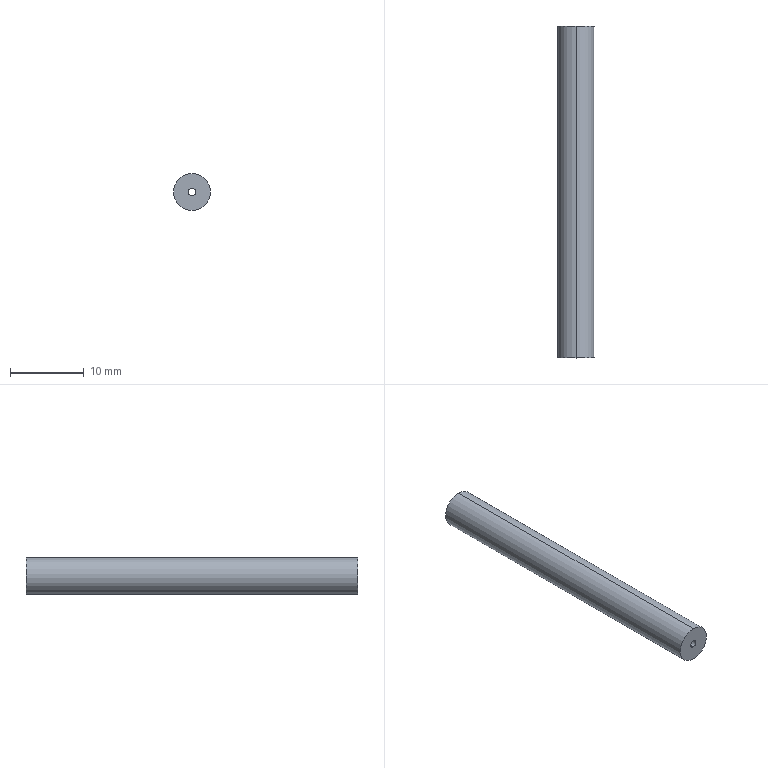Part | SolidWorks | features Extrusion 1, ICE 1 | 1 solid | 9 faces | box 5 x 45 x 5 mm | volume 578.053 mm3 | cylinder 6 | plane 3 | commonest cylinder face diameters 1 x2 3 x2 5 x2
STEP:
#1=CARTESIAN_POINT('',(0.,2.,0.5));
#2=VERTEX_POINT('',#1);
#3=CARTESIAN_POINT('',(0.,2.,-0.5));
#4=VERTEX_POINT('',#3);
#5=CARTESIAN_POINT('',(0.,2.,0.));
#6=DIRECTION('',(0.,-1.,0.));
#7=DIRECTION('',(0.,0.,-1.));
#8=AXIS2_PLACEMENT_3D('',#5,#6,#7);
#9=CIRCLE('',#8,0.5);
#10=EDGE_CURVE('',#2,#4,#9,.T.);
#11=ORIENTED_EDGE('',*,*,#10,.F.);
#12=CARTESIAN_POINT('',(0.,0.,0.5));
#13=VERTEX_POINT('',#12);
#14=CARTESIAN_POINT('',(0.,2.,0.5));
#15=DIRECTION('',(0.,-1.,0.));
#16=VECTOR('',#15,1000.);
#17=LINE('',#14,#16);
#18=EDGE_CURVE('',#2,#13,#17,.T.);
#19=ORIENTED_EDGE('',*,*,#18,.T.);
#20=CARTESIAN_POINT('',(0.,0.,-0.5));
#21=VERTEX_POINT('',#20);
#22=CARTESIAN_POINT('',(0.,0.,0.));
#23=DIRECTION('',(0.,-1.,0.));
#24=DIRECTION('',(0.,0.,-1.));
#25=AXIS2_PLACEMENT_3D('',#22,#23,#24);
#26=CIRCLE('',#25,0.5);
#27=EDGE_CURVE('',#13,#21,#26,.T.);
#28=ORIENTED_EDGE('',*,*,#27,.T.);
#29=CARTESIAN_POINT('',(0.,2.,-0.5));
#30=DIRECTION('',(0.,-1.,0.));
#31=VECTOR('',#30,1000.);
#32=LINE('',#29,#31);
#33=EDGE_CURVE('',#4,#21,#32,.T.);
#34=ORIENTED_EDGE('',*,*,#33,.F.);
#35=EDGE_LOOP('',(#11,#19,#28,#34));
#36=FACE_OUTER_BOUND('',#35,.T.);
#37=CARTESIAN_POINT('',(0.,2.,0.));
#38=DIRECTION('',(0.,-1.,0.));
#39=DIRECTION('',(0.,0.,-1.));
#40=AXIS2_PLACEMENT_3D('',#37,#38,#39);
#41=CYLINDRICAL_SURFACE('',#40,0.5);
#42=ADVANCED_FACE('',(#36),#41,.F.);
#43=CARTESIAN_POINT('',(0.,45.,2.5));
#44=VERTEX_POINT('',#43);
#45=CARTESIAN_POINT('',(0.,45.,-2.5));
#46=VERTEX_POINT('',#45);
#47=CARTESIAN_POINT('',(0.,45.,0.));
#48=DIRECTION('',(0.,1.,0.));
#49=DIRECTION('',(0.,0.,1.));
#50=AXIS2_PLACEMENT_3D('',#47,#48,#49);
#51=CIRCLE('',#50,2.5);
#52=EDGE_CURVE('',#44,#46,#51,.T.);
#53=ORIENTED_EDGE('',*,*,#52,.F.);
#54=CARTESIAN_POINT('',(0.,0.,2.5));
#55=VERTEX_POINT('',#54);
#56=CARTESIAN_POINT('',(0.,45.,2.5));
#57=DIRECTION('',(0.,-1.,0.));
#58=VECTOR('',#57,1000.);
#59=LINE('',#56,#58);
#60=EDGE_CURVE('',#44,#55,#59,.T.);
#61=ORIENTED_EDGE('',*,*,#60,.T.);
#62=CARTESIAN_POINT('',(0.,0.,-2.5));
#63=VERTEX_POINT('',#62);
#64=CARTESIAN_POINT('',(0.,0.,0.));
#65=DIRECTION('',(0.,1.,0.));
#66=DIRECTION('',(0.,0.,1.));
#67=AXIS2_PLACEMENT_3D('',#64,#65,#66);
#68=CIRCLE('',#67,2.5);
#69=EDGE_CURVE('',#55,#63,#68,.T.);
#70=ORIENTED_EDGE('',*,*,#69,.T.);
#71=CARTESIAN_POINT('',(0.,45.,-2.5));
#72=DIRECTION('',(0.,-1.,0.));
#73=VECTOR('',#72,1000.);
#74=LINE('',#71,#73);
#75=EDGE_CURVE('',#46,#63,#74,.T.);
#76=ORIENTED_EDGE('',*,*,#75,.F.);
#77=EDGE_LOOP('',(#53,#61,#70,#76));
#78=FACE_OUTER_BOUND('',#77,.T.);
#79=CARTESIAN_POINT('',(0.,45.,0.));
#80=DIRECTION('',(0.,-1.,0.));
#81=DIRECTION('',(0.,0.,-1.));
#82=AXIS2_PLACEMENT_3D('',#79,#80,#81);
#83=CYLINDRICAL_SURFACE('',#82,2.5);
#84=ADVANCED_FACE('',(#78),#83,.T.);
#85=CARTESIAN_POINT('',(0.,45.,-1.5));
#86=VERTEX_POINT('',#85);
#87=CARTESIAN_POINT('',(0.,45.,1.5));
#88=VERTEX_POINT('',#87);
#89=CARTESIAN_POINT('',(0.,45.,0.));
#90=DIRECTION('',(0.,1.,0.));
#91=DIRECTION('',(0.,0.,1.));
#92=AXIS2_PLACEMENT_3D('',#89,#90,#91);
#93=CIRCLE('',#92,1.5);
#94=EDGE_CURVE('',#86,#88,#93,.T.);
#95=ORIENTED_EDGE('',*,*,#94,.T.);
#96=CARTESIAN_POINT('',(0.,2.,1.5));
#97=VERTEX_POINT('',#96);
#98=CARTESIAN_POINT('',(0.,45.,1.5));
#99=DIRECTION('',(0.,-1.,0.));
#100=VECTOR('',#99,1000.);
#101=LINE('',#98,#100);
#102=EDGE_CURVE('',#88,#97,#101,.T.);
#103=ORIENTED_EDGE('',*,*,#102,.T.);
#104=CARTESIAN_POINT('',(0.,2.,-1.5));
#105=VERTEX_POINT('',#104);
#106=CARTESIAN_POINT('',(0.,2.,0.));
#107=DIRECTION('',(0.,-1.,0.));
#108=DIRECTION('',(0.,0.,-1.));
#109=AXIS2_PLACEMENT_3D('',#106,#107,#108);
#110=CIRCLE('',#109,1.5);
#111=EDGE_CURVE('',#97,#105,#110,.T.);
#112=ORIENTED_EDGE('',*,*,#111,.T.);
#113=CARTESIAN_POINT('',(0.,45.,-1.5));
#114=DIRECTION('',(0.,-1.,0.));
#115=VECTOR('',#114,1000.);
#116=LINE('',#113,#115);
#117=EDGE_CURVE('',#86,#105,#116,.T.);
#118=ORIENTED_EDGE('',*,*,#117,.F.);
#119=EDGE_LOOP('',(#95,#103,#112,#118));
#120=FACE_OUTER_BOUND('',#119,.T.);
#121=CARTESIAN_POINT('',(0.,45.,0.));
#122=DIRECTION('',(0.,-1.,0.));
#123=DIRECTION('',(0.,0.,-1.));
#124=AXIS2_PLACEMENT_3D('',#121,#122,#123);
#125=CYLINDRICAL_SURFACE('',#124,1.5);
#126=ADVANCED_FACE('',(#120),#125,.F.);
#127=ORIENTED_EDGE('',*,*,#102,.F.);
#128=CARTESIAN_POINT('',(0.,45.,0.));
#129=DIRECTION('',(0.,1.,0.));
#130=DIRECTION('',(0.,0.,1.));
#131=AXIS2_PLACEMENT_3D('',#128,#129,#130);
#132=CIRCLE('',#131,1.5);
#133=EDGE_CURVE('',#88,#86,#132,.T.);
#134=ORIENTED_EDGE('',*,*,#133,.T.);
#135=ORIENTED_EDGE('',*,*,#117,.T.);
#136=CARTESIAN_POINT('',(0.,2.,0.));
#137=DIRECTION('',(0.,-1.,0.));
#138=DIRECTION('',(0.,0.,-1.));
#139=AXIS2_PLACEMENT_3D('',#136,#137,#138);
#140=CIRCLE('',#139,1.5);
#141=EDGE_CURVE('',#105,#97,#140,.T.);
#142=ORIENTED_EDGE('',*,*,#141,.T.);
#143=EDGE_LOOP('',(#127,#134,#135,#142));
#144=FACE_OUTER_BOUND('',#143,.T.);
#145=CARTESIAN_POINT('',(0.,45.,0.));
#146=DIRECTION('',(0.,-1.,0.));
#147=DIRECTION('',(0.,0.,-1.));
#148=AXIS2_PLACEMENT_3D('',#145,#146,#147);
#149=CYLINDRICAL_SURFACE('',#148,1.5);
#150=ADVANCED_FACE('',(#144),#149,.F.);
#151=CARTESIAN_POINT('',(0.,45.,0.));
#152=DIRECTION('',(0.,1.,0.));
#153=DIRECTION('',(0.,0.,1.));
#154=AXIS2_PLACEMENT_3D('',#151,#152,#153);
#155=CIRCLE('',#154,2.5);
#156=EDGE_CURVE('',#46,#44,#155,.T.);
#157=ORIENTED_EDGE('',*,*,#156,.T.);
#158=ORIENTED_EDGE('',*,*,#52,.T.);
#159=EDGE_LOOP('',(#157,#158));
#160=FACE_OUTER_BOUND('',#159,.T.);
#161=ORIENTED_EDGE('',*,*,#94,.F.);
#162=ORIENTED_EDGE('',*,*,#133,.F.);
#163=EDGE_LOOP('',(#161,#162));
#164=FACE_BOUND('',#163,.T.);
#165=CARTESIAN_POINT('',(0.,45.,0.));
#166=DIRECTION('',(0.,1.,0.));
#167=DIRECTION('',(0.,0.,1.));
#168=AXIS2_PLACEMENT_3D('',#165,#166,#167);
#169=PLANE('',#168);
#170=ADVANCED_FACE('',(#160,#164),#169,.T.);
#171=CARTESIAN_POINT('',(0.,0.,0.));
#172=DIRECTION('',(0.,1.,0.));
#173=DIRECTION('',(0.,0.,1.));
#174=AXIS2_PLACEMENT_3D('',#171,#172,#173);
#175=CIRCLE('',#174,2.5);
#176=EDGE_CURVE('',#63,#55,#175,.T.);
#177=ORIENTED_EDGE('',*,*,#176,.F.);
#178=ORIENTED_EDGE('',*,*,#69,.F.);
#179=EDGE_LOOP('',(#177,#178));
#180=FACE_OUTER_BOUND('',#179,.T.);
#181=CARTESIAN_POINT('',(0.,0.,0.));
#182=DIRECTION('',(0.,-1.,0.));
#183=DIRECTION('',(0.,0.,-1.));
#184=AXIS2_PLACEMENT_3D('',#181,#182,#183);
#185=CIRCLE('',#184,0.5);
#186=EDGE_CURVE('',#21,#13,#185,.T.);
#187=ORIENTED_EDGE('',*,*,#186,.F.);
#188=ORIENTED_EDGE('',*,*,#27,.F.);
#189=EDGE_LOOP('',(#187,#188));
#190=FACE_BOUND('',#189,.T.);
#191=CARTESIAN_POINT('',(0.,0.,0.));
#192=DIRECTION('',(0.,1.,0.));
#193=DIRECTION('',(0.,0.,1.));
#194=AXIS2_PLACEMENT_3D('',#191,#192,#193);
#195=PLANE('',#194);
#196=ADVANCED_FACE('',(#180,#190),#195,.F.);
#197=ORIENTED_EDGE('',*,*,#60,.F.);
#198=ORIENTED_EDGE('',*,*,#156,.F.);
#199=ORIENTED_EDGE('',*,*,#75,.T.);
#200=ORIENTED_EDGE('',*,*,#176,.T.);
#201=EDGE_LOOP('',(#197,#198,#199,#200));
#202=FACE_OUTER_BOUND('',#201,.T.);
#203=CARTESIAN_POINT('',(0.,45.,0.));
#204=DIRECTION('',(0.,-1.,0.));
#205=DIRECTION('',(0.,0.,-1.));
#206=AXIS2_PLACEMENT_3D('',#203,#204,#205);
#207=CYLINDRICAL_SURFACE('',#206,2.5);
#208=ADVANCED_FACE('',(#202),#207,.T.);
#209=CARTESIAN_POINT('',(0.,2.,0.));
#210=DIRECTION('',(0.,-1.,0.));
#211=DIRECTION('',(0.,0.,-1.));
#212=AXIS2_PLACEMENT_3D('',#209,#210,#211);
#213=CIRCLE('',#212,0.5);
#214=EDGE_CURVE('',#4,#2,#213,.T.);
#215=ORIENTED_EDGE('',*,*,#214,.T.);
#216=ORIENTED_EDGE('',*,*,#10,.T.);
#217=EDGE_LOOP('',(#215,#216));
#218=FACE_BOUND('',#217,.T.);
#219=ORIENTED_EDGE('',*,*,#141,.F.);
#220=ORIENTED_EDGE('',*,*,#111,.F.);
#221=EDGE_LOOP('',(#219,#220));
#222=FACE_OUTER_BOUND('',#221,.T.);
#223=CARTESIAN_POINT('',(0.,2.,0.));
#224=DIRECTION('',(0.,-1.,0.));
#225=DIRECTION('',(0.,0.,-1.));
#226=AXIS2_PLACEMENT_3D('',#223,#224,#225);
#227=PLANE('',#226);
#228=ADVANCED_FACE('',(#218,#222),#227,.F.);
#229=ORIENTED_EDGE('',*,*,#18,.F.);
#230=ORIENTED_EDGE('',*,*,#214,.F.);
#231=ORIENTED_EDGE('',*,*,#33,.T.);
#232=ORIENTED_EDGE('',*,*,#186,.T.);
#233=EDGE_LOOP('',(#229,#230,#231,#232));
#234=FACE_OUTER_BOUND('',#233,.T.);
#235=CARTESIAN_POINT('',(0.,2.,0.));
#236=DIRECTION('',(0.,-1.,0.));
#237=DIRECTION('',(0.,0.,-1.));
#238=AXIS2_PLACEMENT_3D('',#235,#236,#237);
#239=CYLINDRICAL_SURFACE('',#238,0.5);
#240=ADVANCED_FACE('',(#234),#239,.F.);
#241=CLOSED_SHELL('',(#42,#84,#126,#150,#170,#196,#208,#228,#240));
#242=MANIFOLD_SOLID_BREP('',#241);
#243=CARTESIAN_POINT('',(0.,0.,0.));
#244=DIRECTION('',(0.,0.,1.));
#245=DIRECTION('',(1.,0.,0.));
#246=AXIS2_PLACEMENT_3D('',#243,#244,#245);
#247=(LENGTH_UNIT()NAMED_UNIT(*)SI_UNIT(.MILLI.,.METRE.));
#248=UNCERTAINTY_MEASURE_WITH_UNIT(LENGTH_MEASURE(0.00001),#247,'','');
#249=(NAMED_UNIT(*)PLANE_ANGLE_UNIT()SI_UNIT($,.RADIAN.));
#250=(NAMED_UNIT(*)SI_UNIT($,.STERADIAN.)SOLID_ANGLE_UNIT());
#251=(GEOMETRIC_REPRESENTATION_CONTEXT(3)GLOBAL_UNCERTAINTY_ASSIGNED_CONTEXT((#248))GLOBAL_UNIT_ASSIGNED_CONTEXT((#247,#249,#250))REPRESENTATION_CONTEXT('',''));
#252=ADVANCED_BREP_SHAPE_REPRESENTATION('',(#242,#246),#251);